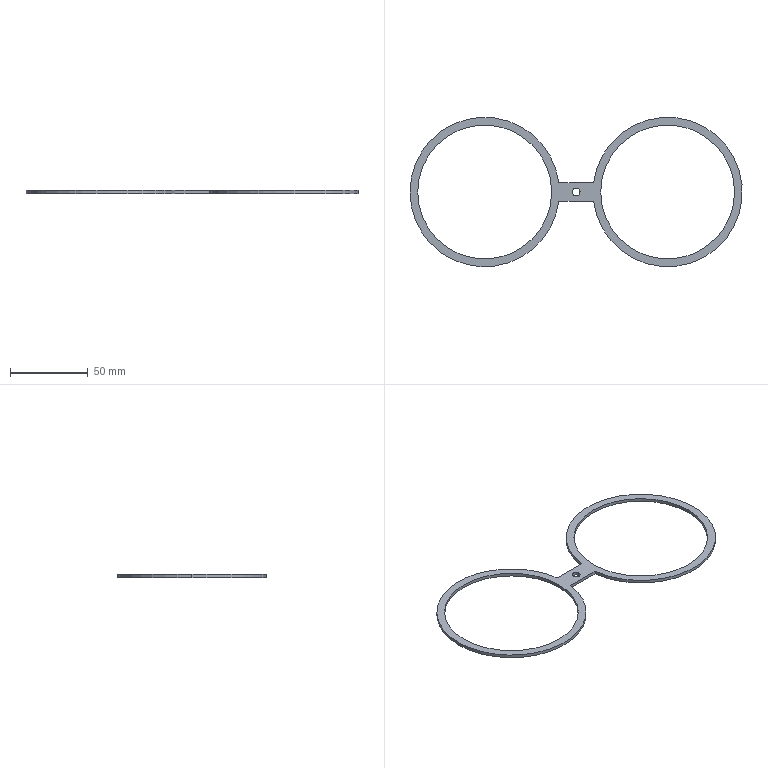Part | SolidWorks | features Extrusion 1 | 1 solid | 13 faces | box 213.58 x 96 x 2 mm | volume 6205 mm3 | cylinder 9 | plane 4 | commonest cylinder face diameters 86 x4 96 x3 5 x2
STEP:
#1=CARTESIAN_POINT('',(56.29,0.,2.));
#2=VERTEX_POINT('',#1);
#3=CARTESIAN_POINT('',(61.29,0.,2.));
#4=VERTEX_POINT('',#3);
#5=CARTESIAN_POINT('',(58.79,0.,2.));
#6=DIRECTION('',(0.,0.,1.));
#7=DIRECTION('',(1.,0.,0.));
#8=AXIS2_PLACEMENT_3D('',#5,#6,#7);
#9=CIRCLE('',#8,2.5);
#10=EDGE_CURVE('',#2,#4,#9,.T.);
#11=ORIENTED_EDGE('',*,*,#10,.T.);
#12=CARTESIAN_POINT('',(61.29,0.,0.));
#13=VERTEX_POINT('',#12);
#14=CARTESIAN_POINT('',(61.29,0.,2.));
#15=DIRECTION('',(0.,0.,-1.));
#16=VECTOR('',#15,1000.);
#17=LINE('',#14,#16);
#18=EDGE_CURVE('',#4,#13,#17,.T.);
#19=ORIENTED_EDGE('',*,*,#18,.T.);
#20=CARTESIAN_POINT('',(56.29,0.,0.));
#21=VERTEX_POINT('',#20);
#22=CARTESIAN_POINT('',(58.79,0.,0.));
#23=DIRECTION('',(0.,0.,1.));
#24=DIRECTION('',(1.,0.,0.));
#25=AXIS2_PLACEMENT_3D('',#22,#23,#24);
#26=CIRCLE('',#25,2.5);
#27=EDGE_CURVE('',#21,#13,#26,.T.);
#28=ORIENTED_EDGE('',*,*,#27,.F.);
#29=CARTESIAN_POINT('',(56.29,0.,2.));
#30=DIRECTION('',(0.,0.,-1.));
#31=VECTOR('',#30,1000.);
#32=LINE('',#29,#31);
#33=EDGE_CURVE('',#2,#21,#32,.T.);
#34=ORIENTED_EDGE('',*,*,#33,.F.);
#35=EDGE_LOOP('',(#11,#19,#28,#34));
#36=FACE_OUTER_BOUND('',#35,.T.);
#37=CARTESIAN_POINT('',(58.79,0.,2.));
#38=DIRECTION('',(0.,0.,-1.));
#39=DIRECTION('',(-1.,0.,0.));
#40=AXIS2_PLACEMENT_3D('',#37,#38,#39);
#41=CYLINDRICAL_SURFACE('',#40,2.5);
#42=ADVANCED_FACE('',(#36),#41,.F.);
#43=CARTESIAN_POINT('',(74.58,0.,2.));
#44=VERTEX_POINT('',#43);
#45=CARTESIAN_POINT('',(160.58,0.,2.));
#46=VERTEX_POINT('',#45);
#47=CARTESIAN_POINT('',(117.58,0.,2.));
#48=DIRECTION('',(0.,0.,1.));
#49=DIRECTION('',(1.,0.,0.));
#50=AXIS2_PLACEMENT_3D('',#47,#48,#49);
#51=CIRCLE('',#50,43.);
#52=EDGE_CURVE('',#44,#46,#51,.T.);
#53=ORIENTED_EDGE('',*,*,#52,.T.);
#54=CARTESIAN_POINT('',(160.58,0.,0.));
#55=VERTEX_POINT('',#54);
#56=CARTESIAN_POINT('',(160.58,0.,2.));
#57=DIRECTION('',(0.,0.,-1.));
#58=VECTOR('',#57,1000.);
#59=LINE('',#56,#58);
#60=EDGE_CURVE('',#46,#55,#59,.T.);
#61=ORIENTED_EDGE('',*,*,#60,.T.);
#62=CARTESIAN_POINT('',(74.58,0.,0.));
#63=VERTEX_POINT('',#62);
#64=CARTESIAN_POINT('',(117.58,0.,0.));
#65=DIRECTION('',(0.,0.,1.));
#66=DIRECTION('',(1.,0.,0.));
#67=AXIS2_PLACEMENT_3D('',#64,#65,#66);
#68=CIRCLE('',#67,43.);
#69=EDGE_CURVE('',#63,#55,#68,.T.);
#70=ORIENTED_EDGE('',*,*,#69,.F.);
#71=CARTESIAN_POINT('',(74.58,0.,2.));
#72=DIRECTION('',(0.,0.,-1.));
#73=VECTOR('',#72,1000.);
#74=LINE('',#71,#73);
#75=EDGE_CURVE('',#44,#63,#74,.T.);
#76=ORIENTED_EDGE('',*,*,#75,.F.);
#77=EDGE_LOOP('',(#53,#61,#70,#76));
#78=FACE_OUTER_BOUND('',#77,.T.);
#79=CARTESIAN_POINT('',(117.58,0.,2.));
#80=DIRECTION('',(0.,0.,-1.));
#81=DIRECTION('',(-1.,0.,0.));
#82=AXIS2_PLACEMENT_3D('',#79,#80,#81);
#83=CYLINDRICAL_SURFACE('',#82,43.);
#84=ADVANCED_FACE('',(#78),#83,.F.);
#85=CARTESIAN_POINT('',(-43.,0.,2.));
#86=VERTEX_POINT('',#85);
#87=CARTESIAN_POINT('',(43.,0.,2.));
#88=VERTEX_POINT('',#87);
#89=CARTESIAN_POINT('',(0.,0.,2.));
#90=DIRECTION('',(0.,0.,1.));
#91=DIRECTION('',(1.,0.,0.));
#92=AXIS2_PLACEMENT_3D('',#89,#90,#91);
#93=CIRCLE('',#92,43.);
#94=EDGE_CURVE('',#86,#88,#93,.T.);
#95=ORIENTED_EDGE('',*,*,#94,.T.);
#96=CARTESIAN_POINT('',(43.,0.,0.));
#97=VERTEX_POINT('',#96);
#98=CARTESIAN_POINT('',(43.,0.,2.));
#99=DIRECTION('',(0.,0.,-1.));
#100=VECTOR('',#99,1000.);
#101=LINE('',#98,#100);
#102=EDGE_CURVE('',#88,#97,#101,.T.);
#103=ORIENTED_EDGE('',*,*,#102,.T.);
#104=CARTESIAN_POINT('',(-43.,0.,0.));
#105=VERTEX_POINT('',#104);
#106=CARTESIAN_POINT('',(0.,0.,0.));
#107=DIRECTION('',(0.,0.,1.));
#108=DIRECTION('',(1.,0.,0.));
#109=AXIS2_PLACEMENT_3D('',#106,#107,#108);
#110=CIRCLE('',#109,43.);
#111=EDGE_CURVE('',#105,#97,#110,.T.);
#112=ORIENTED_EDGE('',*,*,#111,.F.);
#113=CARTESIAN_POINT('',(-43.,0.,2.));
#114=DIRECTION('',(0.,0.,-1.));
#115=VECTOR('',#114,1000.);
#116=LINE('',#113,#115);
#117=EDGE_CURVE('',#86,#105,#116,.T.);
#118=ORIENTED_EDGE('',*,*,#117,.F.);
#119=EDGE_LOOP('',(#95,#103,#112,#118));
#120=FACE_OUTER_BOUND('',#119,.T.);
#121=CARTESIAN_POINT('',(0.,0.,2.));
#122=DIRECTION('',(0.,0.,-1.));
#123=DIRECTION('',(-1.,0.,0.));
#124=AXIS2_PLACEMENT_3D('',#121,#122,#123);
#125=CYLINDRICAL_SURFACE('',#124,43.);
#126=ADVANCED_FACE('',(#120),#125,.F.);
#127=CARTESIAN_POINT('',(-48.,0.,2.));
#128=VERTEX_POINT('',#127);
#129=CARTESIAN_POINT('',(47.621,-6.02,2.));
#130=VERTEX_POINT('',#129);
#131=CARTESIAN_POINT('',(0.,0.,2.));
#132=DIRECTION('',(0.,0.,1.));
#133=DIRECTION('',(1.,0.,0.));
#134=AXIS2_PLACEMENT_3D('',#131,#132,#133);
#135=CIRCLE('',#134,48.);
#136=EDGE_CURVE('',#128,#130,#135,.T.);
#137=ORIENTED_EDGE('',*,*,#136,.F.);
#138=CARTESIAN_POINT('',(-48.,0.,0.));
#139=VERTEX_POINT('',#138);
#140=CARTESIAN_POINT('',(-48.,0.,2.));
#141=DIRECTION('',(0.,0.,-1.));
#142=VECTOR('',#141,1000.);
#143=LINE('',#140,#142);
#144=EDGE_CURVE('',#128,#139,#143,.T.);
#145=ORIENTED_EDGE('',*,*,#144,.T.);
#146=CARTESIAN_POINT('',(47.621,-6.02,0.));
#147=VERTEX_POINT('',#146);
#148=CARTESIAN_POINT('',(0.,0.,0.));
#149=DIRECTION('',(0.,0.,1.));
#150=DIRECTION('',(1.,0.,0.));
#151=AXIS2_PLACEMENT_3D('',#148,#149,#150);
#152=CIRCLE('',#151,48.);
#153=EDGE_CURVE('',#139,#147,#152,.T.);
#154=ORIENTED_EDGE('',*,*,#153,.T.);
#155=CARTESIAN_POINT('',(47.621,-6.02,2.));
#156=DIRECTION('',(0.,0.,-1.));
#157=VECTOR('',#156,1000.);
#158=LINE('',#155,#157);
#159=EDGE_CURVE('',#130,#147,#158,.T.);
#160=ORIENTED_EDGE('',*,*,#159,.F.);
#161=EDGE_LOOP('',(#137,#145,#154,#160));
#162=FACE_OUTER_BOUND('',#161,.T.);
#163=CARTESIAN_POINT('',(0.,0.,2.));
#164=DIRECTION('',(0.,0.,-1.));
#165=DIRECTION('',(-1.,0.,0.));
#166=AXIS2_PLACEMENT_3D('',#163,#164,#165);
#167=CYLINDRICAL_SURFACE('',#166,48.);
#168=ADVANCED_FACE('',(#162),#167,.T.);
#169=ORIENTED_EDGE('',*,*,#52,.F.);
#170=CARTESIAN_POINT('',(117.58,0.,2.));
#171=DIRECTION('',(0.,0.,1.));
#172=DIRECTION('',(1.,0.,0.));
#173=AXIS2_PLACEMENT_3D('',#170,#171,#172);
#174=CIRCLE('',#173,43.);
#175=EDGE_CURVE('',#46,#44,#174,.T.);
#176=ORIENTED_EDGE('',*,*,#175,.F.);
#177=EDGE_LOOP('',(#169,#176));
#178=FACE_BOUND('',#177,.T.);
#179=CARTESIAN_POINT('',(69.959,-6.02,2.));
#180=VERTEX_POINT('',#179);
#181=CARTESIAN_POINT('',(69.962,6.045,2.));
#182=VERTEX_POINT('',#181);
#183=CARTESIAN_POINT('',(117.58,0.,2.));
#184=DIRECTION('',(0.,0.,1.));
#185=DIRECTION('',(1.,0.,0.));
#186=AXIS2_PLACEMENT_3D('',#183,#184,#185);
#187=CIRCLE('',#186,48.);
#188=EDGE_CURVE('',#180,#182,#187,.T.);
#189=ORIENTED_EDGE('',*,*,#188,.T.);
#190=CARTESIAN_POINT('',(47.618,6.045,2.));
#191=VERTEX_POINT('',#190);
#192=CARTESIAN_POINT('',(47.618,6.045,2.));
#193=DIRECTION('',(-1.,0.,0.));
#194=VECTOR('',#193,1000.);
#195=LINE('',#192,#194);
#196=EDGE_CURVE('',#182,#191,#195,.T.);
#197=ORIENTED_EDGE('',*,*,#196,.T.);
#198=CARTESIAN_POINT('',(0.,0.,2.));
#199=DIRECTION('',(0.,0.,1.));
#200=DIRECTION('',(1.,0.,0.));
#201=AXIS2_PLACEMENT_3D('',#198,#199,#200);
#202=CIRCLE('',#201,48.);
#203=EDGE_CURVE('',#191,#128,#202,.T.);
#204=ORIENTED_EDGE('',*,*,#203,.T.);
#205=ORIENTED_EDGE('',*,*,#136,.T.);
#206=CARTESIAN_POINT('',(69.959,-6.02,2.));
#207=DIRECTION('',(1.,0.,0.));
#208=VECTOR('',#207,1000.);
#209=LINE('',#206,#208);
#210=EDGE_CURVE('',#130,#180,#209,.T.);
#211=ORIENTED_EDGE('',*,*,#210,.T.);
#212=EDGE_LOOP('',(#189,#197,#204,#205,#211));
#213=FACE_OUTER_BOUND('',#212,.T.);
#214=ORIENTED_EDGE('',*,*,#94,.F.);
#215=CARTESIAN_POINT('',(0.,0.,2.));
#216=DIRECTION('',(0.,0.,1.));
#217=DIRECTION('',(1.,0.,0.));
#218=AXIS2_PLACEMENT_3D('',#215,#216,#217);
#219=CIRCLE('',#218,43.);
#220=EDGE_CURVE('',#88,#86,#219,.T.);
#221=ORIENTED_EDGE('',*,*,#220,.F.);
#222=EDGE_LOOP('',(#214,#221));
#223=FACE_BOUND('',#222,.T.);
#224=ORIENTED_EDGE('',*,*,#10,.F.);
#225=CARTESIAN_POINT('',(58.79,0.,2.));
#226=DIRECTION('',(0.,0.,1.));
#227=DIRECTION('',(1.,0.,0.));
#228=AXIS2_PLACEMENT_3D('',#225,#226,#227);
#229=CIRCLE('',#228,2.5);
#230=EDGE_CURVE('',#4,#2,#229,.T.);
#231=ORIENTED_EDGE('',*,*,#230,.F.);
#232=EDGE_LOOP('',(#224,#231));
#233=FACE_BOUND('',#232,.T.);
#234=CARTESIAN_POINT('',(117.58,0.,2.));
#235=DIRECTION('',(0.,0.,1.));
#236=DIRECTION('',(1.,0.,0.));
#237=AXIS2_PLACEMENT_3D('',#234,#235,#236);
#238=PLANE('',#237);
#239=ADVANCED_FACE('',(#178,#213,#223,#233),#238,.T.);
#240=CARTESIAN_POINT('',(69.959,-6.02,0.));
#241=VERTEX_POINT('',#240);
#242=CARTESIAN_POINT('',(69.962,6.045,0.));
#243=VERTEX_POINT('',#242);
#244=CARTESIAN_POINT('',(117.58,0.,0.));
#245=DIRECTION('',(0.,0.,1.));
#246=DIRECTION('',(1.,0.,0.));
#247=AXIS2_PLACEMENT_3D('',#244,#245,#246);
#248=CIRCLE('',#247,48.);
#249=EDGE_CURVE('',#241,#243,#248,.T.);
#250=ORIENTED_EDGE('',*,*,#249,.F.);
#251=CARTESIAN_POINT('',(69.959,-6.02,0.));
#252=DIRECTION('',(1.,0.,0.));
#253=VECTOR('',#252,1000.);
#254=LINE('',#251,#253);
#255=EDGE_CURVE('',#147,#241,#254,.T.);
#256=ORIENTED_EDGE('',*,*,#255,.F.);
#257=ORIENTED_EDGE('',*,*,#153,.F.);
#258=CARTESIAN_POINT('',(47.618,6.045,0.));
#259=VERTEX_POINT('',#258);
#260=CARTESIAN_POINT('',(0.,0.,0.));
#261=DIRECTION('',(0.,0.,1.));
#262=DIRECTION('',(1.,0.,0.));
#263=AXIS2_PLACEMENT_3D('',#260,#261,#262);
#264=CIRCLE('',#263,48.);
#265=EDGE_CURVE('',#259,#139,#264,.T.);
#266=ORIENTED_EDGE('',*,*,#265,.F.);
#267=CARTESIAN_POINT('',(47.618,6.045,0.));
#268=DIRECTION('',(-1.,0.,0.));
#269=VECTOR('',#268,1000.);
#270=LINE('',#267,#269);
#271=EDGE_CURVE('',#243,#259,#270,.T.);
#272=ORIENTED_EDGE('',*,*,#271,.F.);
#273=EDGE_LOOP('',(#250,#256,#257,#266,#272));
#274=FACE_OUTER_BOUND('',#273,.T.);
#275=ORIENTED_EDGE('',*,*,#111,.T.);
#276=CARTESIAN_POINT('',(0.,0.,0.));
#277=DIRECTION('',(0.,0.,1.));
#278=DIRECTION('',(1.,0.,0.));
#279=AXIS2_PLACEMENT_3D('',#276,#277,#278);
#280=CIRCLE('',#279,43.);
#281=EDGE_CURVE('',#97,#105,#280,.T.);
#282=ORIENTED_EDGE('',*,*,#281,.T.);
#283=EDGE_LOOP('',(#275,#282));
#284=FACE_BOUND('',#283,.T.);
#285=ORIENTED_EDGE('',*,*,#69,.T.);
#286=CARTESIAN_POINT('',(117.58,0.,0.));
#287=DIRECTION('',(0.,0.,1.));
#288=DIRECTION('',(1.,0.,0.));
#289=AXIS2_PLACEMENT_3D('',#286,#287,#288);
#290=CIRCLE('',#289,43.);
#291=EDGE_CURVE('',#55,#63,#290,.T.);
#292=ORIENTED_EDGE('',*,*,#291,.T.);
#293=EDGE_LOOP('',(#285,#292));
#294=FACE_BOUND('',#293,.T.);
#295=ORIENTED_EDGE('',*,*,#27,.T.);
#296=CARTESIAN_POINT('',(58.79,0.,0.));
#297=DIRECTION('',(0.,0.,1.));
#298=DIRECTION('',(1.,0.,0.));
#299=AXIS2_PLACEMENT_3D('',#296,#297,#298);
#300=CIRCLE('',#299,2.5);
#301=EDGE_CURVE('',#13,#21,#300,.T.);
#302=ORIENTED_EDGE('',*,*,#301,.T.);
#303=EDGE_LOOP('',(#295,#302));
#304=FACE_BOUND('',#303,.T.);
#305=CARTESIAN_POINT('',(117.58,0.,0.));
#306=DIRECTION('',(0.,0.,1.));
#307=DIRECTION('',(1.,0.,0.));
#308=AXIS2_PLACEMENT_3D('',#305,#306,#307);
#309=PLANE('',#308);
#310=ADVANCED_FACE('',(#274,#284,#294,#304),#309,.F.);
#311=ORIENTED_EDGE('',*,*,#249,.T.);
#312=CARTESIAN_POINT('',(69.962,6.045,2.));
#313=DIRECTION('',(0.,0.,-1.));
#314=VECTOR('',#313,1000.);
#315=LINE('',#312,#314);
#316=EDGE_CURVE('',#182,#243,#315,.T.);
#317=ORIENTED_EDGE('',*,*,#316,.F.);
#318=ORIENTED_EDGE('',*,*,#188,.F.);
#319=CARTESIAN_POINT('',(69.959,-6.02,2.));
#320=DIRECTION('',(0.,0.,-1.));
#321=VECTOR('',#320,1000.);
#322=LINE('',#319,#321);
#323=EDGE_CURVE('',#180,#241,#322,.T.);
#324=ORIENTED_EDGE('',*,*,#323,.T.);
#325=EDGE_LOOP('',(#311,#317,#318,#324));
#326=FACE_OUTER_BOUND('',#325,.T.);
#327=CARTESIAN_POINT('',(117.58,0.,2.));
#328=DIRECTION('',(0.,0.,-1.));
#329=DIRECTION('',(-1.,0.,0.));
#330=AXIS2_PLACEMENT_3D('',#327,#328,#329);
#331=CYLINDRICAL_SURFACE('',#330,48.);
#332=ADVANCED_FACE('',(#326),#331,.T.);
#333=ORIENTED_EDGE('',*,*,#271,.T.);
#334=CARTESIAN_POINT('',(47.618,6.045,2.));
#335=DIRECTION('',(0.,0.,-1.));
#336=VECTOR('',#335,1000.);
#337=LINE('',#334,#336);
#338=EDGE_CURVE('',#191,#259,#337,.T.);
#339=ORIENTED_EDGE('',*,*,#338,.F.);
#340=ORIENTED_EDGE('',*,*,#196,.F.);
#341=ORIENTED_EDGE('',*,*,#316,.T.);
#342=EDGE_LOOP('',(#333,#339,#340,#341));
#343=FACE_OUTER_BOUND('',#342,.T.);
#344=CARTESIAN_POINT('',(47.618,6.045,2.));
#345=DIRECTION('',(0.,-1.,0.));
#346=DIRECTION('',(0.,0.,-1.));
#347=AXIS2_PLACEMENT_3D('',#344,#345,#346);
#348=PLANE('',#347);
#349=ADVANCED_FACE('',(#343),#348,.F.);
#350=ORIENTED_EDGE('',*,*,#144,.F.);
#351=ORIENTED_EDGE('',*,*,#203,.F.);
#352=ORIENTED_EDGE('',*,*,#338,.T.);
#353=ORIENTED_EDGE('',*,*,#265,.T.);
#354=EDGE_LOOP('',(#350,#351,#352,#353));
#355=FACE_OUTER_BOUND('',#354,.T.);
#356=CARTESIAN_POINT('',(0.,0.,2.));
#357=DIRECTION('',(0.,0.,-1.));
#358=DIRECTION('',(-1.,0.,0.));
#359=AXIS2_PLACEMENT_3D('',#356,#357,#358);
#360=CYLINDRICAL_SURFACE('',#359,48.);
#361=ADVANCED_FACE('',(#355),#360,.T.);
#362=ORIENTED_EDGE('',*,*,#255,.T.);
#363=ORIENTED_EDGE('',*,*,#323,.F.);
#364=ORIENTED_EDGE('',*,*,#210,.F.);
#365=ORIENTED_EDGE('',*,*,#159,.T.);
#366=EDGE_LOOP('',(#362,#363,#364,#365));
#367=FACE_OUTER_BOUND('',#366,.T.);
#368=CARTESIAN_POINT('',(69.959,-6.02,2.));
#369=DIRECTION('',(0.,1.,0.));
#370=DIRECTION('',(0.,0.,1.));
#371=AXIS2_PLACEMENT_3D('',#368,#369,#370);
#372=PLANE('',#371);
#373=ADVANCED_FACE('',(#367),#372,.F.);
#374=ORIENTED_EDGE('',*,*,#102,.F.);
#375=ORIENTED_EDGE('',*,*,#220,.T.);
#376=ORIENTED_EDGE('',*,*,#117,.T.);
#377=ORIENTED_EDGE('',*,*,#281,.F.);
#378=EDGE_LOOP('',(#374,#375,#376,#377));
#379=FACE_OUTER_BOUND('',#378,.T.);
#380=CARTESIAN_POINT('',(0.,0.,2.));
#381=DIRECTION('',(0.,0.,-1.));
#382=DIRECTION('',(-1.,0.,0.));
#383=AXIS2_PLACEMENT_3D('',#380,#381,#382);
#384=CYLINDRICAL_SURFACE('',#383,43.);
#385=ADVANCED_FACE('',(#379),#384,.F.);
#386=ORIENTED_EDGE('',*,*,#60,.F.);
#387=ORIENTED_EDGE('',*,*,#175,.T.);
#388=ORIENTED_EDGE('',*,*,#75,.T.);
#389=ORIENTED_EDGE('',*,*,#291,.F.);
#390=EDGE_LOOP('',(#386,#387,#388,#389));
#391=FACE_OUTER_BOUND('',#390,.T.);
#392=CARTESIAN_POINT('',(117.58,0.,2.));
#393=DIRECTION('',(0.,0.,-1.));
#394=DIRECTION('',(-1.,0.,0.));
#395=AXIS2_PLACEMENT_3D('',#392,#393,#394);
#396=CYLINDRICAL_SURFACE('',#395,43.);
#397=ADVANCED_FACE('',(#391),#396,.F.);
#398=ORIENTED_EDGE('',*,*,#18,.F.);
#399=ORIENTED_EDGE('',*,*,#230,.T.);
#400=ORIENTED_EDGE('',*,*,#33,.T.);
#401=ORIENTED_EDGE('',*,*,#301,.F.);
#402=EDGE_LOOP('',(#398,#399,#400,#401));
#403=FACE_OUTER_BOUND('',#402,.T.);
#404=CARTESIAN_POINT('',(58.79,0.,2.));
#405=DIRECTION('',(0.,0.,-1.));
#406=DIRECTION('',(-1.,0.,0.));
#407=AXIS2_PLACEMENT_3D('',#404,#405,#406);
#408=CYLINDRICAL_SURFACE('',#407,2.5);
#409=ADVANCED_FACE('',(#403),#408,.F.);
#410=CLOSED_SHELL('',(#42,#84,#126,#168,#239,#310,#332,#349,#361,#373,#385,#397,#409));
#411=MANIFOLD_SOLID_BREP('',#410);
#412=CARTESIAN_POINT('',(0.,0.,0.));
#413=DIRECTION('',(0.,0.,1.));
#414=DIRECTION('',(1.,0.,0.));
#415=AXIS2_PLACEMENT_3D('',#412,#413,#414);
#416=(LENGTH_UNIT()NAMED_UNIT(*)SI_UNIT(.MILLI.,.METRE.));
#417=UNCERTAINTY_MEASURE_WITH_UNIT(LENGTH_MEASURE(0.00001),#416,'','');
#418=(NAMED_UNIT(*)PLANE_ANGLE_UNIT()SI_UNIT($,.RADIAN.));
#419=(NAMED_UNIT(*)SI_UNIT($,.STERADIAN.)SOLID_ANGLE_UNIT());
#420=(GEOMETRIC_REPRESENTATION_CONTEXT(3)GLOBAL_UNCERTAINTY_ASSIGNED_CONTEXT((#417))GLOBAL_UNIT_ASSIGNED_CONTEXT((#416,#418,#419))REPRESENTATION_CONTEXT('',''));
#421=ADVANCED_BREP_SHAPE_REPRESENTATION('',(#411,#415),#420);